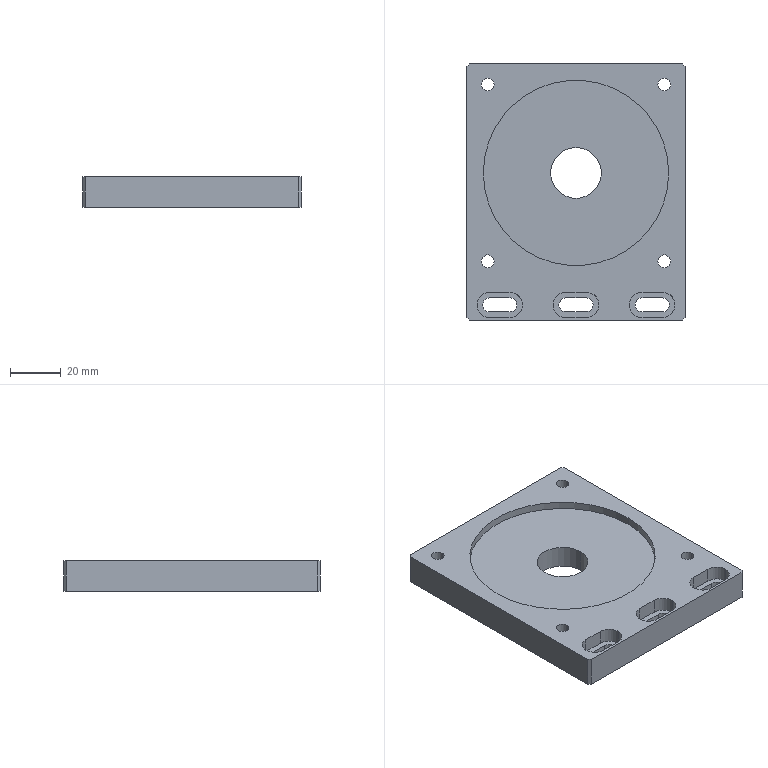Part | STEP file | Flat belt motor mounting plate | 1 solid | 56 faces | box 86 x 101 x 12 mm | volume 83890 mm3 | cylinder 30 | plane 26 | commonest cylinder face diameters 5.5 x9 10 x9 5 x8 20 x2 73 x2